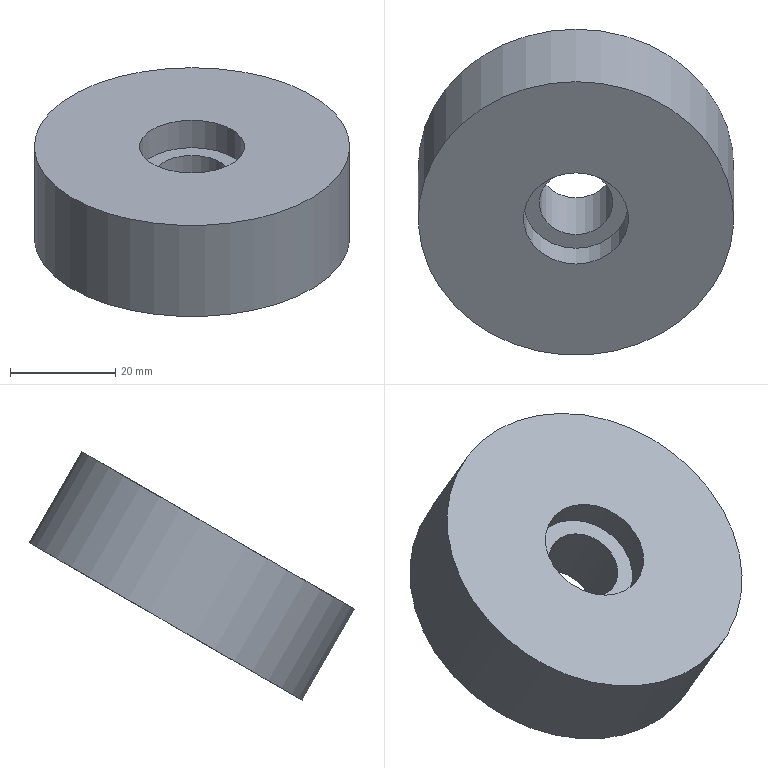Part | NX | features solid 2 | 1 solid | 6 faces | box 60 x 61.962 x 47.321 mm | volume 52509 mm3 | cylinder 3 | plane 3 | commonest cylinder face diameters 14 x1 20 x1 60 x1
STEP:
#1=CARTESIAN_POINT('',(-305.,-464.032,275.836));
#2=VERTEX_POINT('',#1);
#3=CARTESIAN_POINT('',(-305.,-490.013,260.836));
#4=DIRECTION('',(0.,-0.5,0.866));
#5=DIRECTION('',(0.,0.866,0.5));
#6=AXIS2_PLACEMENT_3D('',#3,#4,#5);
#7=CIRCLE('',#6,30.);
#8=EDGE_CURVE('',#2,#2,#7,.T.);
#9=ORIENTED_EDGE('',*,*,#8,.F.);
#10=EDGE_LOOP('',(#9));
#11=FACE_BOUND('',#10,.T.);
#12=CARTESIAN_POINT('',(-305.,-454.032,258.516));
#13=VERTEX_POINT('',#12);
#14=CARTESIAN_POINT('',(-305.,-480.013,243.516));
#15=DIRECTION('',(0.,-0.5,0.866));
#16=DIRECTION('',(0.,0.866,0.5));
#17=AXIS2_PLACEMENT_3D('',#14,#15,#16);
#18=CIRCLE('',#17,30.);
#19=EDGE_CURVE('',#13,#13,#18,.T.);
#20=ORIENTED_EDGE('',*,*,#19,.T.);
#21=EDGE_LOOP('',(#20));
#22=FACE_BOUND('',#21,.T.);
#23=CARTESIAN_POINT('',(-305.,-490.013,260.836));
#24=DIRECTION('',(0.,0.5,-0.866));
#25=DIRECTION('',(0.,0.866,0.5));
#26=AXIS2_PLACEMENT_3D('',#23,#24,#25);
#27=CYLINDRICAL_SURFACE('',#26,30.);
#28=ADVANCED_FACE('',(#11,#22),#27,.T.);
#29=CARTESIAN_POINT('',(-305.,-481.353,265.836));
#30=VERTEX_POINT('',#29);
#31=CARTESIAN_POINT('',(-305.,-490.013,260.836));
#32=DIRECTION('',(0.,-0.5,0.866));
#33=DIRECTION('',(0.,0.866,0.5));
#34=AXIS2_PLACEMENT_3D('',#31,#32,#33);
#35=CIRCLE('',#34,10.);
#36=EDGE_CURVE('',#30,#30,#35,.T.);
#37=ORIENTED_EDGE('',*,*,#36,.F.);
#38=EDGE_LOOP('',(#37));
#39=FACE_BOUND('',#38,.T.);
#40=ORIENTED_EDGE('',*,*,#8,.T.);
#41=EDGE_LOOP('',(#40));
#42=FACE_BOUND('',#41,.T.);
#43=CARTESIAN_POINT('',(-305.,-490.013,260.836));
#44=DIRECTION('',(0.,0.5,-0.866));
#45=DIRECTION('',(0.,0.866,0.5));
#46=AXIS2_PLACEMENT_3D('',#43,#44,#45);
#47=PLANE('',#46);
#48=ADVANCED_FACE('',(#39,#42),#47,.F.);
#49=CARTESIAN_POINT('',(-305.,-473.951,247.016));
#50=VERTEX_POINT('',#49);
#51=CARTESIAN_POINT('',(-305.,-480.013,243.516));
#52=DIRECTION('',(0.,-0.5,0.866));
#53=DIRECTION('',(0.,0.866,0.5));
#54=AXIS2_PLACEMENT_3D('',#51,#52,#53);
#55=CIRCLE('',#54,7.);
#56=EDGE_CURVE('',#50,#50,#55,.T.);
#57=ORIENTED_EDGE('',*,*,#56,.T.);
#58=EDGE_LOOP('',(#57));
#59=FACE_BOUND('',#58,.T.);
#60=ORIENTED_EDGE('',*,*,#19,.F.);
#61=EDGE_LOOP('',(#60));
#62=FACE_BOUND('',#61,.T.);
#63=CARTESIAN_POINT('',(-305.,-480.013,243.516));
#64=DIRECTION('',(0.,0.5,-0.866));
#65=DIRECTION('',(0.,0.866,0.5));
#66=AXIS2_PLACEMENT_3D('',#63,#64,#65);
#67=PLANE('',#66);
#68=ADVANCED_FACE('',(#59,#62),#67,.T.);
#69=CARTESIAN_POINT('',(-305.,-495.673,250.64));
#70=VERTEX_POINT('',#69);
#71=CARTESIAN_POINT('',(-305.,-487.013,255.64));
#72=DIRECTION('',(0.,0.5,-0.866));
#73=DIRECTION('',(0.,-0.866,-0.5));
#74=AXIS2_PLACEMENT_3D('',#71,#72,#73);
#75=CIRCLE('',#74,10.);
#76=EDGE_CURVE('',#70,#70,#75,.T.);
#77=ORIENTED_EDGE('',*,*,#76,.T.);
#78=EDGE_LOOP('',(#77));
#79=FACE_BOUND('',#78,.T.);
#80=ORIENTED_EDGE('',*,*,#36,.T.);
#81=EDGE_LOOP('',(#80));
#82=FACE_BOUND('',#81,.T.);
#83=CARTESIAN_POINT('',(-305.,-487.013,255.64));
#84=DIRECTION('',(0.,-0.5,0.866));
#85=DIRECTION('',(0.,-0.866,-0.5));
#86=AXIS2_PLACEMENT_3D('',#83,#84,#85);
#87=CYLINDRICAL_SURFACE('',#86,10.);
#88=ADVANCED_FACE('',(#79,#82),#87,.F.);
#89=ORIENTED_EDGE('',*,*,#56,.F.);
#90=EDGE_LOOP('',(#89));
#91=FACE_BOUND('',#90,.T.);
#92=CARTESIAN_POINT('',(-305.,-480.951,259.14));
#93=VERTEX_POINT('',#92);
#94=CARTESIAN_POINT('',(-305.,-487.013,255.64));
#95=DIRECTION('',(0.,-0.5,0.866));
#96=DIRECTION('',(0.,0.866,0.5));
#97=AXIS2_PLACEMENT_3D('',#94,#95,#96);
#98=CIRCLE('',#97,7.);
#99=EDGE_CURVE('',#93,#93,#98,.F.);
#100=ORIENTED_EDGE('',*,*,#99,.F.);
#101=EDGE_LOOP('',(#100));
#102=FACE_BOUND('',#101,.T.);
#103=CARTESIAN_POINT('',(-305.,-473.013,231.392));
#104=DIRECTION('',(0.,-0.5,0.866));
#105=DIRECTION('',(0.,-0.866,-0.5));
#106=AXIS2_PLACEMENT_3D('',#103,#104,#105);
#107=CYLINDRICAL_SURFACE('',#106,7.);
#108=ADVANCED_FACE('',(#91,#102),#107,.F.);
#109=ORIENTED_EDGE('',*,*,#99,.T.);
#110=EDGE_LOOP('',(#109));
#111=FACE_BOUND('',#110,.T.);
#112=ORIENTED_EDGE('',*,*,#76,.F.);
#113=EDGE_LOOP('',(#112));
#114=FACE_BOUND('',#113,.T.);
#115=CARTESIAN_POINT('',(-305.,-487.013,255.64));
#116=DIRECTION('',(0.,0.5,-0.866));
#117=DIRECTION('',(0.,0.866,0.5));
#118=AXIS2_PLACEMENT_3D('',#115,#116,#117);
#119=PLANE('',#118);
#120=ADVANCED_FACE('',(#111,#114),#119,.F.);
#121=CLOSED_SHELL('',(#28,#48,#68,#88,#108,#120));
#122=MANIFOLD_SOLID_BREP('',#121);
#123=(LENGTH_UNIT()NAMED_UNIT(*)SI_UNIT(.MILLI.,.METRE.));
#124=UNCERTAINTY_MEASURE_WITH_UNIT(LENGTH_MEASURE(0.00001),#123,'','');
#125=(NAMED_UNIT(*)PLANE_ANGLE_UNIT()SI_UNIT($,.RADIAN.));
#126=(NAMED_UNIT(*)SI_UNIT($,.STERADIAN.)SOLID_ANGLE_UNIT());
#127=(GEOMETRIC_REPRESENTATION_CONTEXT(3)GLOBAL_UNCERTAINTY_ASSIGNED_CONTEXT((#124))GLOBAL_UNIT_ASSIGNED_CONTEXT((#123,#125,#126))REPRESENTATION_CONTEXT('',''));
#128=ADVANCED_BREP_SHAPE_REPRESENTATION('',(#122),#127);